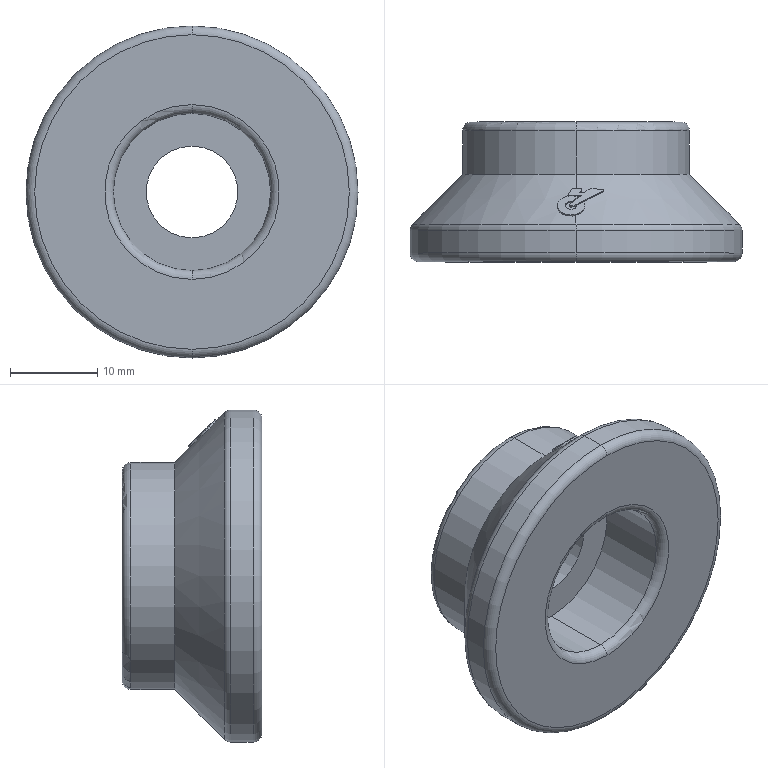Part | NX | features solid 2 | 1 solid | 53 faces | box 38 x 16 x 38 mm | volume 9635 mm3 | spline 21 | cylinder 10 | cone 8 | torus 8 | plane 6 | commonest cylinder face diameters 10.5 x2 18 x2 26 x2 38 x2 4.141 x1 6.578 x1